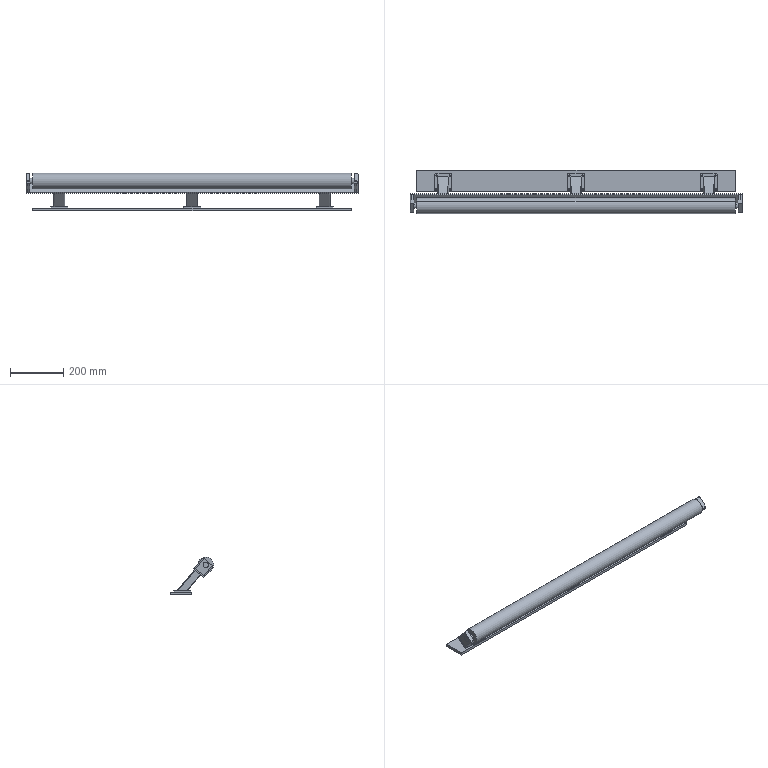Part | SolidWorks | features CompositeCurve 1 | 9 solids | 168 faces | box 1250 x 163.16 x 142.786 mm | volume 4866204 mm3 | plane 80 | cylinder 64 | spline 24 | commonest cylinder face diameters 5.2 x24 10 x18 4.2 x8 20 x8 24 x4 60 x2